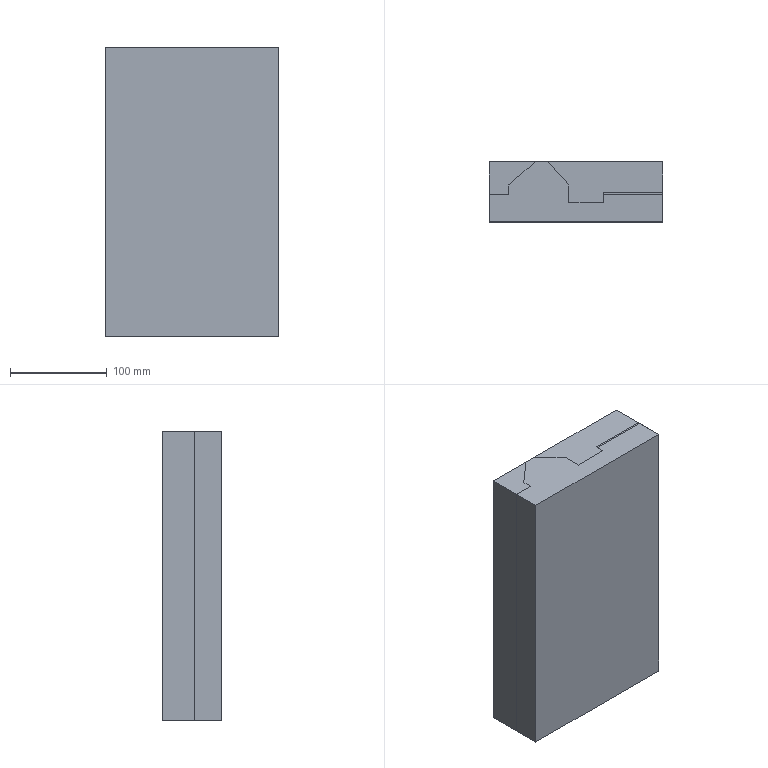CAM job | NX | 3-axis milling | part box 180 x 62 x 300 mm | stock box 180 x 62 x 300 mm
Tools:
number,name,description,diameter,corner_radius,flute_length,length,flutes
0,D21R0.8圆鼻飞刀,Milling Tool-5 Parameters,25.0,0.8,50.0,50.0,2
0,D50飞刀,Milling Tool-5 Parameters,63.0,0.0,100.0,100.0,2
15,D17R0.8圆鼻飞刀,Milling Tool-5 Parameters,17.0,0.8,60.0,60.0,2
Operations:
program,operation,operation_type,tool,method,geometry_group,spindle_rpm,surface_speed,feed_per_tooth,feed_cut,feed_plunge,cut_length_mm,path_length_mm,cut_time_min,machine_time_min
1,型腔铣_COPY,CavityMilling,D50飞刀,METHOD,WORKPIECE---A,1500.0,117.0,0.6667,2000.0,100.0,98127.437,138306.117,53.498,57.516
1,型腔铣,CavityMilling,D21R0.8圆鼻飞刀,METHOD,WORKPIECE---A,1500.0,117.0,0.6667,2000.0,100.0,416935.97,491031.732,217.228,224.637
1,定轴曲面加工,SurfaceContour,D17R0.8圆鼻飞刀,METHOD,MCS---A,2000.0,106.0,0.5,2000.0,70.0,147650.93,148066.933,73.831,73.873
.NC,等高外形,ZLevelMilling,D21R0.8圆鼻飞刀,METHOD,MCS---A,1500.0,117.0,0.6667,2000.0,80.0,11046.4,11179.812,5.614,5.627
.NC_1,飞平面_1,VolumeBased25DMillingOperation,D21R0.8圆鼻飞刀,METHOD,MCS---A,1500.0,117.0,0.6667,2000.0,80.0,17817.638,18262.787,8.961,9.006
.NC_1,飞平面,VolumeBased25DMillingOperation,D21R0.8圆鼻飞刀,METHOD,MCS---A,3000.0,282.0,0.0,1500.0,80.0,1914.548,2524.876,1.282,1.343